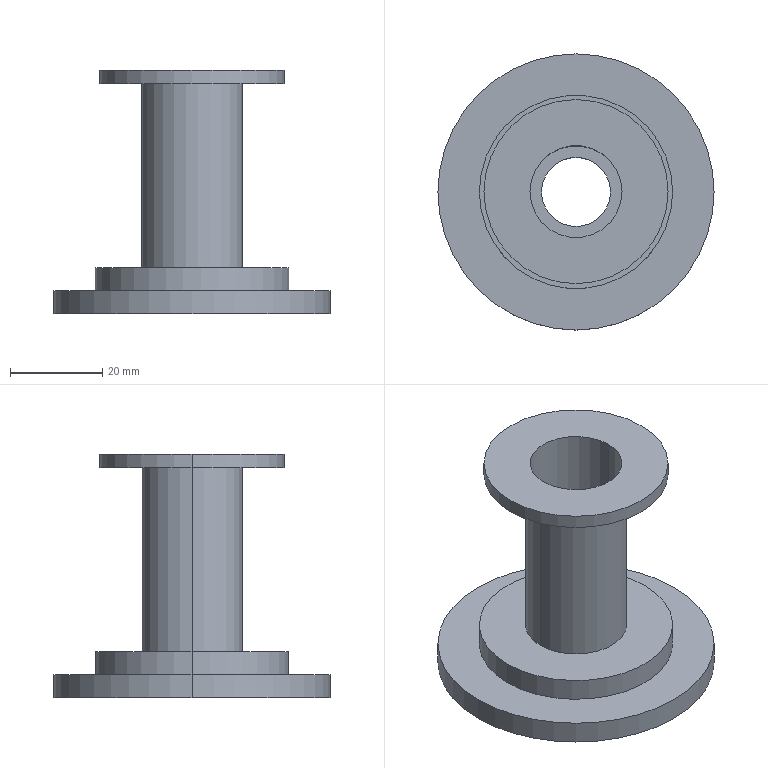Part | STEP file | Base | 1 solid | 18 faces | box 60 x 60 x 53 mm | volume 24076 mm3 | cylinder 12 | plane 6 | commonest cylinder face diameters 15 x2 20 x2 22 x2 40 x2 42 x2 60 x2
STEP:
#1=CARTESIAN_POINT('',(20.,0.,53.));
#2=VERTEX_POINT('',#1);
#3=CARTESIAN_POINT('',(-20.,0.,53.));
#4=VERTEX_POINT('',#3);
#5=CARTESIAN_POINT('',(0.,0.,53.));
#6=DIRECTION('',(0.,0.,1.));
#7=DIRECTION('',(1.,0.,0.));
#8=AXIS2_PLACEMENT_3D('',#5,#6,#7);
#9=CIRCLE('',#8,20.);
#10=EDGE_CURVE('',#2,#4,#9,.T.);
#11=ORIENTED_EDGE('',*,*,#10,.F.);
#12=CARTESIAN_POINT('',(20.,0.,50.));
#13=VERTEX_POINT('',#12);
#14=CARTESIAN_POINT('',(20.,0.,53.));
#15=DIRECTION('',(0.,0.,-1.));
#16=VECTOR('',#15,1000.);
#17=LINE('',#14,#16);
#18=EDGE_CURVE('',#2,#13,#17,.T.);
#19=ORIENTED_EDGE('',*,*,#18,.T.);
#20=CARTESIAN_POINT('',(-20.,0.,50.));
#21=VERTEX_POINT('',#20);
#22=CARTESIAN_POINT('',(0.,0.,50.));
#23=DIRECTION('',(0.,0.,1.));
#24=DIRECTION('',(1.,0.,0.));
#25=AXIS2_PLACEMENT_3D('',#22,#23,#24);
#26=CIRCLE('',#25,20.);
#27=EDGE_CURVE('',#13,#21,#26,.T.);
#28=ORIENTED_EDGE('',*,*,#27,.T.);
#29=CARTESIAN_POINT('',(-20.,0.,53.));
#30=DIRECTION('',(0.,0.,-1.));
#31=VECTOR('',#30,1000.);
#32=LINE('',#29,#31);
#33=EDGE_CURVE('',#4,#21,#32,.T.);
#34=ORIENTED_EDGE('',*,*,#33,.F.);
#35=EDGE_LOOP('',(#11,#19,#28,#34));
#36=FACE_OUTER_BOUND('',#35,.T.);
#37=CARTESIAN_POINT('',(0.,0.,53.));
#38=DIRECTION('',(0.,0.,-1.));
#39=DIRECTION('',(-1.,0.,0.));
#40=AXIS2_PLACEMENT_3D('',#37,#38,#39);
#41=CYLINDRICAL_SURFACE('',#40,20.);
#42=ADVANCED_FACE('',(#36),#41,.T.);
#43=CARTESIAN_POINT('',(11.,0.,50.));
#44=VERTEX_POINT('',#43);
#45=CARTESIAN_POINT('',(-11.,0.,50.));
#46=VERTEX_POINT('',#45);
#47=CARTESIAN_POINT('',(0.,0.,50.));
#48=DIRECTION('',(0.,0.,1.));
#49=DIRECTION('',(1.,0.,0.));
#50=AXIS2_PLACEMENT_3D('',#47,#48,#49);
#51=CIRCLE('',#50,11.);
#52=EDGE_CURVE('',#44,#46,#51,.T.);
#53=ORIENTED_EDGE('',*,*,#52,.F.);
#54=CARTESIAN_POINT('',(11.,0.,10.));
#55=VERTEX_POINT('',#54);
#56=CARTESIAN_POINT('',(11.,0.,50.));
#57=DIRECTION('',(0.,0.,-1.));
#58=VECTOR('',#57,1000.);
#59=LINE('',#56,#58);
#60=EDGE_CURVE('',#44,#55,#59,.T.);
#61=ORIENTED_EDGE('',*,*,#60,.T.);
#62=CARTESIAN_POINT('',(-11.,0.,10.));
#63=VERTEX_POINT('',#62);
#64=CARTESIAN_POINT('',(0.,0.,10.));
#65=DIRECTION('',(0.,0.,1.));
#66=DIRECTION('',(1.,0.,0.));
#67=AXIS2_PLACEMENT_3D('',#64,#65,#66);
#68=CIRCLE('',#67,11.);
#69=EDGE_CURVE('',#55,#63,#68,.T.);
#70=ORIENTED_EDGE('',*,*,#69,.T.);
#71=CARTESIAN_POINT('',(-11.,0.,50.));
#72=DIRECTION('',(0.,0.,-1.));
#73=VECTOR('',#72,1000.);
#74=LINE('',#71,#73);
#75=EDGE_CURVE('',#46,#63,#74,.T.);
#76=ORIENTED_EDGE('',*,*,#75,.F.);
#77=EDGE_LOOP('',(#53,#61,#70,#76));
#78=FACE_OUTER_BOUND('',#77,.T.);
#79=CARTESIAN_POINT('',(0.,0.,50.));
#80=DIRECTION('',(0.,0.,-1.));
#81=DIRECTION('',(-1.,0.,0.));
#82=AXIS2_PLACEMENT_3D('',#79,#80,#81);
#83=CYLINDRICAL_SURFACE('',#82,11.);
#84=ADVANCED_FACE('',(#78),#83,.T.);
#85=CARTESIAN_POINT('',(-7.5,0.,0.));
#86=VERTEX_POINT('',#85);
#87=CARTESIAN_POINT('',(7.5,0.,0.));
#88=VERTEX_POINT('',#87);
#89=CARTESIAN_POINT('',(0.,0.,0.));
#90=DIRECTION('',(0.,0.,1.));
#91=DIRECTION('',(1.,0.,0.));
#92=AXIS2_PLACEMENT_3D('',#89,#90,#91);
#93=CIRCLE('',#92,7.5);
#94=EDGE_CURVE('',#86,#88,#93,.T.);
#95=ORIENTED_EDGE('',*,*,#94,.F.);
#96=CARTESIAN_POINT('',(-7.5,0.,5.));
#97=VERTEX_POINT('',#96);
#98=CARTESIAN_POINT('',(-7.5,0.,0.));
#99=DIRECTION('',(0.,0.,1.));
#100=VECTOR('',#99,1000.);
#101=LINE('',#98,#100);
#102=EDGE_CURVE('',#86,#97,#101,.T.);
#103=ORIENTED_EDGE('',*,*,#102,.T.);
#104=CARTESIAN_POINT('',(7.5,0.,5.));
#105=VERTEX_POINT('',#104);
#106=CARTESIAN_POINT('',(0.,0.,5.));
#107=DIRECTION('',(0.,0.,1.));
#108=DIRECTION('',(1.,0.,0.));
#109=AXIS2_PLACEMENT_3D('',#106,#107,#108);
#110=CIRCLE('',#109,7.5);
#111=EDGE_CURVE('',#97,#105,#110,.T.);
#112=ORIENTED_EDGE('',*,*,#111,.T.);
#113=CARTESIAN_POINT('',(7.5,0.,0.));
#114=DIRECTION('',(0.,0.,1.));
#115=VECTOR('',#114,1000.);
#116=LINE('',#113,#115);
#117=EDGE_CURVE('',#88,#105,#116,.T.);
#118=ORIENTED_EDGE('',*,*,#117,.F.);
#119=EDGE_LOOP('',(#95,#103,#112,#118));
#120=FACE_OUTER_BOUND('',#119,.T.);
#121=CARTESIAN_POINT('',(0.,0.,0.));
#122=DIRECTION('',(0.,0.,1.));
#123=DIRECTION('',(1.,0.,0.));
#124=AXIS2_PLACEMENT_3D('',#121,#122,#123);
#125=CYLINDRICAL_SURFACE('',#124,7.5);
#126=ADVANCED_FACE('',(#120),#125,.F.);
#127=CARTESIAN_POINT('',(-10.,0.,53.));
#128=VERTEX_POINT('',#127);
#129=CARTESIAN_POINT('',(10.,0.,53.));
#130=VERTEX_POINT('',#129);
#131=CARTESIAN_POINT('',(0.,0.,53.));
#132=DIRECTION('',(0.,0.,1.));
#133=DIRECTION('',(1.,0.,0.));
#134=AXIS2_PLACEMENT_3D('',#131,#132,#133);
#135=CIRCLE('',#134,10.);
#136=EDGE_CURVE('',#128,#130,#135,.T.);
#137=ORIENTED_EDGE('',*,*,#136,.T.);
#138=CARTESIAN_POINT('',(10.,0.,5.));
#139=VERTEX_POINT('',#138);
#140=CARTESIAN_POINT('',(10.,0.,10.));
#141=DIRECTION('',(0.,0.,-1.));
#142=VECTOR('',#141,1000.);
#143=LINE('',#140,#142);
#144=EDGE_CURVE('',#130,#139,#143,.T.);
#145=ORIENTED_EDGE('',*,*,#144,.T.);
#146=CARTESIAN_POINT('',(-10.,0.,5.));
#147=VERTEX_POINT('',#146);
#148=CARTESIAN_POINT('',(0.,0.,5.));
#149=DIRECTION('',(0.,0.,-1.));
#150=DIRECTION('',(1.,0.,0.));
#151=AXIS2_PLACEMENT_3D('',#148,#149,#150);
#152=CIRCLE('',#151,10.);
#153=EDGE_CURVE('',#139,#147,#152,.T.);
#154=ORIENTED_EDGE('',*,*,#153,.T.);
#155=CARTESIAN_POINT('',(-10.,0.,10.));
#156=DIRECTION('',(0.,0.,-1.));
#157=VECTOR('',#156,1000.);
#158=LINE('',#155,#157);
#159=EDGE_CURVE('',#128,#147,#158,.T.);
#160=ORIENTED_EDGE('',*,*,#159,.F.);
#161=EDGE_LOOP('',(#137,#145,#154,#160));
#162=FACE_OUTER_BOUND('',#161,.T.);
#163=CARTESIAN_POINT('',(0.,0.,10.));
#164=DIRECTION('',(0.,0.,-1.));
#165=DIRECTION('',(-1.,0.,0.));
#166=AXIS2_PLACEMENT_3D('',#163,#164,#165);
#167=CYLINDRICAL_SURFACE('',#166,10.);
#168=ADVANCED_FACE('',(#162),#167,.F.);
#169=CARTESIAN_POINT('',(21.,0.,10.));
#170=VERTEX_POINT('',#169);
#171=CARTESIAN_POINT('',(-21.,0.,10.));
#172=VERTEX_POINT('',#171);
#173=CARTESIAN_POINT('',(0.,0.,10.));
#174=DIRECTION('',(0.,0.,1.));
#175=DIRECTION('',(1.,0.,0.));
#176=AXIS2_PLACEMENT_3D('',#173,#174,#175);
#177=CIRCLE('',#176,21.);
#178=EDGE_CURVE('',#170,#172,#177,.T.);
#179=ORIENTED_EDGE('',*,*,#178,.F.);
#180=CARTESIAN_POINT('',(21.,0.,5.));
#181=VERTEX_POINT('',#180);
#182=CARTESIAN_POINT('',(21.,0.,10.));
#183=DIRECTION('',(0.,0.,-1.));
#184=VECTOR('',#183,1000.);
#185=LINE('',#182,#184);
#186=EDGE_CURVE('',#170,#181,#185,.T.);
#187=ORIENTED_EDGE('',*,*,#186,.T.);
#188=CARTESIAN_POINT('',(-21.,0.,5.));
#189=VERTEX_POINT('',#188);
#190=CARTESIAN_POINT('',(0.,0.,5.));
#191=DIRECTION('',(0.,0.,1.));
#192=DIRECTION('',(1.,0.,0.));
#193=AXIS2_PLACEMENT_3D('',#190,#191,#192);
#194=CIRCLE('',#193,21.);
#195=EDGE_CURVE('',#181,#189,#194,.T.);
#196=ORIENTED_EDGE('',*,*,#195,.T.);
#197=CARTESIAN_POINT('',(-21.,0.,10.));
#198=DIRECTION('',(0.,0.,-1.));
#199=VECTOR('',#198,1000.);
#200=LINE('',#197,#199);
#201=EDGE_CURVE('',#172,#189,#200,.T.);
#202=ORIENTED_EDGE('',*,*,#201,.F.);
#203=EDGE_LOOP('',(#179,#187,#196,#202));
#204=FACE_OUTER_BOUND('',#203,.T.);
#205=CARTESIAN_POINT('',(0.,0.,10.));
#206=DIRECTION('',(0.,0.,-1.));
#207=DIRECTION('',(-1.,0.,0.));
#208=AXIS2_PLACEMENT_3D('',#205,#206,#207);
#209=CYLINDRICAL_SURFACE('',#208,21.);
#210=ADVANCED_FACE('',(#204),#209,.T.);
#211=CARTESIAN_POINT('',(30.,0.,5.));
#212=VERTEX_POINT('',#211);
#213=CARTESIAN_POINT('',(-30.,0.,5.));
#214=VERTEX_POINT('',#213);
#215=CARTESIAN_POINT('',(0.,0.,5.));
#216=DIRECTION('',(0.,0.,1.));
#217=DIRECTION('',(1.,0.,0.));
#218=AXIS2_PLACEMENT_3D('',#215,#216,#217);
#219=CIRCLE('',#218,30.);
#220=EDGE_CURVE('',#212,#214,#219,.T.);
#221=ORIENTED_EDGE('',*,*,#220,.F.);
#222=CARTESIAN_POINT('',(30.,0.,0.));
#223=VERTEX_POINT('',#222);
#224=CARTESIAN_POINT('',(30.,0.,5.));
#225=DIRECTION('',(0.,0.,-1.));
#226=VECTOR('',#225,1000.);
#227=LINE('',#224,#226);
#228=EDGE_CURVE('',#212,#223,#227,.T.);
#229=ORIENTED_EDGE('',*,*,#228,.T.);
#230=CARTESIAN_POINT('',(-30.,0.,0.));
#231=VERTEX_POINT('',#230);
#232=CARTESIAN_POINT('',(0.,0.,0.));
#233=DIRECTION('',(0.,0.,1.));
#234=DIRECTION('',(1.,0.,0.));
#235=AXIS2_PLACEMENT_3D('',#232,#233,#234);
#236=CIRCLE('',#235,30.);
#237=EDGE_CURVE('',#223,#231,#236,.T.);
#238=ORIENTED_EDGE('',*,*,#237,.T.);
#239=CARTESIAN_POINT('',(-30.,0.,5.));
#240=DIRECTION('',(0.,0.,-1.));
#241=VECTOR('',#240,1000.);
#242=LINE('',#239,#241);
#243=EDGE_CURVE('',#214,#231,#242,.T.);
#244=ORIENTED_EDGE('',*,*,#243,.F.);
#245=EDGE_LOOP('',(#221,#229,#238,#244));
#246=FACE_OUTER_BOUND('',#245,.T.);
#247=CARTESIAN_POINT('',(0.,0.,5.));
#248=DIRECTION('',(0.,0.,-1.));
#249=DIRECTION('',(-1.,0.,0.));
#250=AXIS2_PLACEMENT_3D('',#247,#248,#249);
#251=CYLINDRICAL_SURFACE('',#250,30.);
#252=ADVANCED_FACE('',(#246),#251,.T.);
#253=CARTESIAN_POINT('',(0.,0.,10.));
#254=DIRECTION('',(0.,0.,1.));
#255=DIRECTION('',(1.,0.,0.));
#256=AXIS2_PLACEMENT_3D('',#253,#254,#255);
#257=CIRCLE('',#256,21.);
#258=EDGE_CURVE('',#172,#170,#257,.T.);
#259=ORIENTED_EDGE('',*,*,#258,.T.);
#260=ORIENTED_EDGE('',*,*,#178,.T.);
#261=EDGE_LOOP('',(#259,#260));
#262=FACE_OUTER_BOUND('',#261,.T.);
#263=CARTESIAN_POINT('',(0.,0.,10.));
#264=DIRECTION('',(0.,0.,1.));
#265=DIRECTION('',(1.,0.,0.));
#266=AXIS2_PLACEMENT_3D('',#263,#264,#265);
#267=CIRCLE('',#266,11.);
#268=EDGE_CURVE('',#63,#55,#267,.T.);
#269=ORIENTED_EDGE('',*,*,#268,.F.);
#270=ORIENTED_EDGE('',*,*,#69,.F.);
#271=EDGE_LOOP('',(#269,#270));
#272=FACE_BOUND('',#271,.T.);
#273=CARTESIAN_POINT('',(0.,0.,10.));
#274=DIRECTION('',(0.,0.,1.));
#275=DIRECTION('',(1.,0.,0.));
#276=AXIS2_PLACEMENT_3D('',#273,#274,#275);
#277=PLANE('',#276);
#278=ADVANCED_FACE('',(#262,#272),#277,.T.);
#279=ORIENTED_EDGE('',*,*,#228,.F.);
#280=CARTESIAN_POINT('',(0.,0.,5.));
#281=DIRECTION('',(0.,0.,1.));
#282=DIRECTION('',(1.,0.,0.));
#283=AXIS2_PLACEMENT_3D('',#280,#281,#282);
#284=CIRCLE('',#283,30.);
#285=EDGE_CURVE('',#214,#212,#284,.T.);
#286=ORIENTED_EDGE('',*,*,#285,.F.);
#287=ORIENTED_EDGE('',*,*,#243,.T.);
#288=CARTESIAN_POINT('',(0.,0.,0.));
#289=DIRECTION('',(0.,0.,1.));
#290=DIRECTION('',(1.,0.,0.));
#291=AXIS2_PLACEMENT_3D('',#288,#289,#290);
#292=CIRCLE('',#291,30.);
#293=EDGE_CURVE('',#231,#223,#292,.T.);
#294=ORIENTED_EDGE('',*,*,#293,.T.);
#295=EDGE_LOOP('',(#279,#286,#287,#294));
#296=FACE_OUTER_BOUND('',#295,.T.);
#297=CARTESIAN_POINT('',(0.,0.,5.));
#298=DIRECTION('',(0.,0.,-1.));
#299=DIRECTION('',(-1.,0.,0.));
#300=AXIS2_PLACEMENT_3D('',#297,#298,#299);
#301=CYLINDRICAL_SURFACE('',#300,30.);
#302=ADVANCED_FACE('',(#296),#301,.T.);
#303=CARTESIAN_POINT('',(0.,0.,5.));
#304=DIRECTION('',(0.,0.,1.));
#305=DIRECTION('',(1.,0.,0.));
#306=AXIS2_PLACEMENT_3D('',#303,#304,#305);
#307=CIRCLE('',#306,21.);
#308=EDGE_CURVE('',#189,#181,#307,.T.);
#309=ORIENTED_EDGE('',*,*,#308,.F.);
#310=ORIENTED_EDGE('',*,*,#195,.F.);
#311=EDGE_LOOP('',(#309,#310));
#312=FACE_BOUND('',#311,.T.);
#313=ORIENTED_EDGE('',*,*,#285,.T.);
#314=ORIENTED_EDGE('',*,*,#220,.T.);
#315=EDGE_LOOP('',(#313,#314));
#316=FACE_OUTER_BOUND('',#315,.T.);
#317=CARTESIAN_POINT('',(0.,0.,5.));
#318=DIRECTION('',(0.,0.,1.));
#319=DIRECTION('',(1.,0.,0.));
#320=AXIS2_PLACEMENT_3D('',#317,#318,#319);
#321=PLANE('',#320);
#322=ADVANCED_FACE('',(#312,#316),#321,.T.);
#323=CARTESIAN_POINT('',(0.,0.,0.));
#324=DIRECTION('',(0.,0.,1.));
#325=DIRECTION('',(1.,0.,0.));
#326=AXIS2_PLACEMENT_3D('',#323,#324,#325);
#327=CIRCLE('',#326,7.5);
#328=EDGE_CURVE('',#88,#86,#327,.T.);
#329=ORIENTED_EDGE('',*,*,#328,.T.);
#330=ORIENTED_EDGE('',*,*,#94,.T.);
#331=EDGE_LOOP('',(#329,#330));
#332=FACE_BOUND('',#331,.T.);
#333=ORIENTED_EDGE('',*,*,#293,.F.);
#334=ORIENTED_EDGE('',*,*,#237,.F.);
#335=EDGE_LOOP('',(#333,#334));
#336=FACE_OUTER_BOUND('',#335,.T.);
#337=CARTESIAN_POINT('',(0.,0.,0.));
#338=DIRECTION('',(0.,0.,1.));
#339=DIRECTION('',(1.,0.,0.));
#340=AXIS2_PLACEMENT_3D('',#337,#338,#339);
#341=PLANE('',#340);
#342=ADVANCED_FACE('',(#332,#336),#341,.F.);
#343=ORIENTED_EDGE('',*,*,#186,.F.);
#344=ORIENTED_EDGE('',*,*,#258,.F.);
#345=ORIENTED_EDGE('',*,*,#201,.T.);
#346=ORIENTED_EDGE('',*,*,#308,.T.);
#347=EDGE_LOOP('',(#343,#344,#345,#346));
#348=FACE_OUTER_BOUND('',#347,.T.);
#349=CARTESIAN_POINT('',(0.,0.,10.));
#350=DIRECTION('',(0.,0.,-1.));
#351=DIRECTION('',(-1.,0.,0.));
#352=AXIS2_PLACEMENT_3D('',#349,#350,#351);
#353=CYLINDRICAL_SURFACE('',#352,21.);
#354=ADVANCED_FACE('',(#348),#353,.T.);
#355=ORIENTED_EDGE('',*,*,#144,.F.);
#356=CARTESIAN_POINT('',(0.,0.,53.));
#357=DIRECTION('',(0.,0.,1.));
#358=DIRECTION('',(1.,0.,0.));
#359=AXIS2_PLACEMENT_3D('',#356,#357,#358);
#360=CIRCLE('',#359,10.);
#361=EDGE_CURVE('',#130,#128,#360,.T.);
#362=ORIENTED_EDGE('',*,*,#361,.T.);
#363=ORIENTED_EDGE('',*,*,#159,.T.);
#364=CARTESIAN_POINT('',(0.,0.,5.));
#365=DIRECTION('',(0.,0.,-1.));
#366=DIRECTION('',(1.,0.,0.));
#367=AXIS2_PLACEMENT_3D('',#364,#365,#366);
#368=CIRCLE('',#367,10.);
#369=EDGE_CURVE('',#147,#139,#368,.T.);
#370=ORIENTED_EDGE('',*,*,#369,.T.);
#371=EDGE_LOOP('',(#355,#362,#363,#370));
#372=FACE_OUTER_BOUND('',#371,.T.);
#373=CARTESIAN_POINT('',(0.,0.,10.));
#374=DIRECTION('',(0.,0.,-1.));
#375=DIRECTION('',(-1.,0.,0.));
#376=AXIS2_PLACEMENT_3D('',#373,#374,#375);
#377=CYLINDRICAL_SURFACE('',#376,10.);
#378=ADVANCED_FACE('',(#372),#377,.F.);
#379=CARTESIAN_POINT('',(0.,0.,5.));
#380=DIRECTION('',(0.,0.,1.));
#381=DIRECTION('',(1.,0.,0.));
#382=AXIS2_PLACEMENT_3D('',#379,#380,#381);
#383=CIRCLE('',#382,7.5);
#384=EDGE_CURVE('',#105,#97,#383,.T.);
#385=ORIENTED_EDGE('',*,*,#384,.F.);
#386=ORIENTED_EDGE('',*,*,#111,.F.);
#387=EDGE_LOOP('',(#385,#386));
#388=FACE_BOUND('',#387,.T.);
#389=ORIENTED_EDGE('',*,*,#369,.F.);
#390=ORIENTED_EDGE('',*,*,#153,.F.);
#391=EDGE_LOOP('',(#389,#390));
#392=FACE_OUTER_BOUND('',#391,.T.);
#393=CARTESIAN_POINT('',(0.,0.,5.));
#394=DIRECTION('',(0.,0.,1.));
#395=DIRECTION('',(1.,0.,0.));
#396=AXIS2_PLACEMENT_3D('',#393,#394,#395);
#397=PLANE('',#396);
#398=ADVANCED_FACE('',(#388,#392),#397,.T.);
#399=ORIENTED_EDGE('',*,*,#102,.F.);
#400=ORIENTED_EDGE('',*,*,#328,.F.);
#401=ORIENTED_EDGE('',*,*,#117,.T.);
#402=ORIENTED_EDGE('',*,*,#384,.T.);
#403=EDGE_LOOP('',(#399,#400,#401,#402));
#404=FACE_OUTER_BOUND('',#403,.T.);
#405=CARTESIAN_POINT('',(0.,0.,0.));
#406=DIRECTION('',(0.,0.,1.));
#407=DIRECTION('',(1.,0.,0.));
#408=AXIS2_PLACEMENT_3D('',#405,#406,#407);
#409=CYLINDRICAL_SURFACE('',#408,7.5);
#410=ADVANCED_FACE('',(#404),#409,.F.);
#411=ORIENTED_EDGE('',*,*,#60,.F.);
#412=CARTESIAN_POINT('',(0.,0.,50.));
#413=DIRECTION('',(0.,0.,1.));
#414=DIRECTION('',(1.,0.,0.));
#415=AXIS2_PLACEMENT_3D('',#412,#413,#414);
#416=CIRCLE('',#415,11.);
#417=EDGE_CURVE('',#46,#44,#416,.T.);
#418=ORIENTED_EDGE('',*,*,#417,.F.);
#419=ORIENTED_EDGE('',*,*,#75,.T.);
#420=ORIENTED_EDGE('',*,*,#268,.T.);
#421=EDGE_LOOP('',(#411,#418,#419,#420));
#422=FACE_OUTER_BOUND('',#421,.T.);
#423=CARTESIAN_POINT('',(0.,0.,50.));
#424=DIRECTION('',(0.,0.,-1.));
#425=DIRECTION('',(-1.,0.,0.));
#426=AXIS2_PLACEMENT_3D('',#423,#424,#425);
#427=CYLINDRICAL_SURFACE('',#426,11.);
#428=ADVANCED_FACE('',(#422),#427,.T.);
#429=CARTESIAN_POINT('',(0.,0.,53.));
#430=DIRECTION('',(0.,0.,1.));
#431=DIRECTION('',(1.,0.,0.));
#432=AXIS2_PLACEMENT_3D('',#429,#430,#431);
#433=CIRCLE('',#432,20.);
#434=EDGE_CURVE('',#4,#2,#433,.T.);
#435=ORIENTED_EDGE('',*,*,#434,.T.);
#436=ORIENTED_EDGE('',*,*,#10,.T.);
#437=EDGE_LOOP('',(#435,#436));
#438=FACE_OUTER_BOUND('',#437,.T.);
#439=ORIENTED_EDGE('',*,*,#136,.F.);
#440=ORIENTED_EDGE('',*,*,#361,.F.);
#441=EDGE_LOOP('',(#439,#440));
#442=FACE_BOUND('',#441,.T.);
#443=CARTESIAN_POINT('',(0.,0.,53.));
#444=DIRECTION('',(0.,0.,1.));
#445=DIRECTION('',(1.,0.,0.));
#446=AXIS2_PLACEMENT_3D('',#443,#444,#445);
#447=PLANE('',#446);
#448=ADVANCED_FACE('',(#438,#442),#447,.T.);
#449=ORIENTED_EDGE('',*,*,#417,.T.);
#450=ORIENTED_EDGE('',*,*,#52,.T.);
#451=EDGE_LOOP('',(#449,#450));
#452=FACE_BOUND('',#451,.T.);
#453=CARTESIAN_POINT('',(0.,0.,50.));
#454=DIRECTION('',(0.,0.,1.));
#455=DIRECTION('',(1.,0.,0.));
#456=AXIS2_PLACEMENT_3D('',#453,#454,#455);
#457=CIRCLE('',#456,20.);
#458=EDGE_CURVE('',#21,#13,#457,.T.);
#459=ORIENTED_EDGE('',*,*,#458,.F.);
#460=ORIENTED_EDGE('',*,*,#27,.F.);
#461=EDGE_LOOP('',(#459,#460));
#462=FACE_OUTER_BOUND('',#461,.T.);
#463=CARTESIAN_POINT('',(0.,0.,50.));
#464=DIRECTION('',(0.,0.,1.));
#465=DIRECTION('',(1.,0.,0.));
#466=AXIS2_PLACEMENT_3D('',#463,#464,#465);
#467=PLANE('',#466);
#468=ADVANCED_FACE('',(#452,#462),#467,.F.);
#469=ORIENTED_EDGE('',*,*,#18,.F.);
#470=ORIENTED_EDGE('',*,*,#434,.F.);
#471=ORIENTED_EDGE('',*,*,#33,.T.);
#472=ORIENTED_EDGE('',*,*,#458,.T.);
#473=EDGE_LOOP('',(#469,#470,#471,#472));
#474=FACE_OUTER_BOUND('',#473,.T.);
#475=CARTESIAN_POINT('',(0.,0.,53.));
#476=DIRECTION('',(0.,0.,-1.));
#477=DIRECTION('',(-1.,0.,0.));
#478=AXIS2_PLACEMENT_3D('',#475,#476,#477);
#479=CYLINDRICAL_SURFACE('',#478,20.);
#480=ADVANCED_FACE('',(#474),#479,.T.);
#481=CLOSED_SHELL('',(#42,#84,#126,#168,#210,#252,#278,#302,#322,#342,#354,#378,#398,#410,#428,#448,#468,#480));
#482=MANIFOLD_SOLID_BREP('',#481);
#483=CARTESIAN_POINT('',(0.,0.,0.));
#484=DIRECTION('',(0.,0.,1.));
#485=DIRECTION('',(1.,0.,0.));
#486=AXIS2_PLACEMENT_3D('',#483,#484,#485);
#487=(LENGTH_UNIT()NAMED_UNIT(*)SI_UNIT(.MILLI.,.METRE.));
#488=UNCERTAINTY_MEASURE_WITH_UNIT(LENGTH_MEASURE(0.00001),#487,'','');
#489=(NAMED_UNIT(*)PLANE_ANGLE_UNIT()SI_UNIT($,.RADIAN.));
#490=(NAMED_UNIT(*)SI_UNIT($,.STERADIAN.)SOLID_ANGLE_UNIT());
#491=(GEOMETRIC_REPRESENTATION_CONTEXT(3)GLOBAL_UNCERTAINTY_ASSIGNED_CONTEXT((#488))GLOBAL_UNIT_ASSIGNED_CONTEXT((#487,#489,#490))REPRESENTATION_CONTEXT('',''));
#492=ADVANCED_BREP_SHAPE_REPRESENTATION('',(#482,#486),#491);